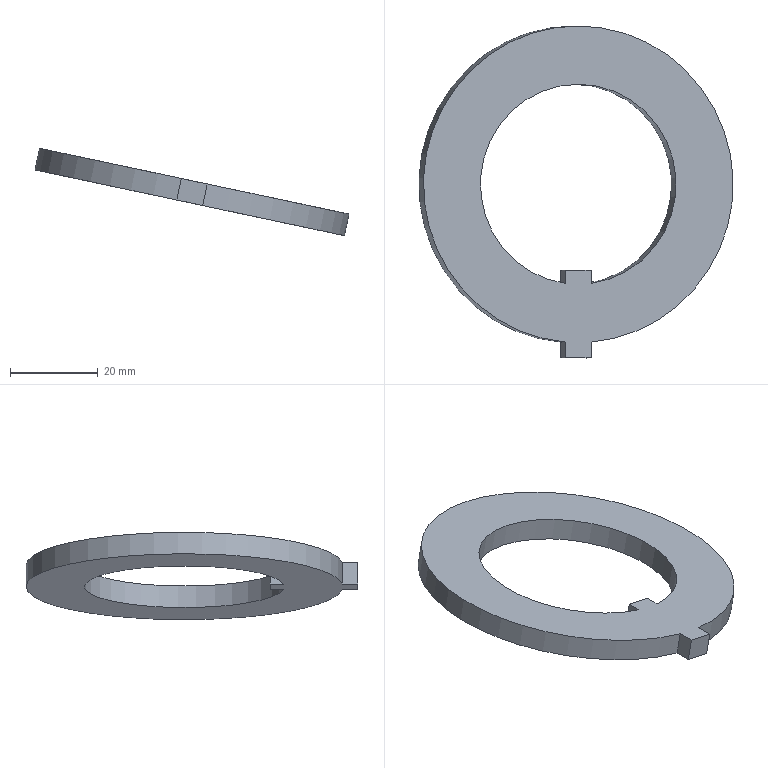Part | STEP file | HL4GZ-1.862.566 (lock washer) | 1 solid | 10 faces | box 71.466 x 75.5 x 19.86 mm | volume 12429 mm3 | plane 8 | cylinder 2 | commonest cylinder face diameters 45.5 x1 72 x1
STEP:
#1=CARTESIAN_POINT('',(0.,0.,0.));
#2=DIRECTION('',(0.,0.,1.));
#3=DIRECTION('',(1.,0.,0.));
#4=AXIS2_PLACEMENT_3D('',#1,#2,#3);
#5=CARTESIAN_POINT('',(1982.907,-35.875,-340.395));
#6=VERTEX_POINT('',#5);
#7=CARTESIAN_POINT('',(1983.947,-35.875,-335.504));
#8=VERTEX_POINT('',#7);
#9=CARTESIAN_POINT('',(1983.947,-35.875,-335.504));
#10=DIRECTION('',(0.2079,0.,0.9781));
#11=VECTOR('',#10,1.);
#12=LINE('',#9,#11);
#13=CARTESIAN_POINT('',(1983.947,-19.5,-335.504));
#14=DIRECTION('',(0.9781,0.,-0.2079));
#15=DIRECTION('',(0.,-1.,0.));
#16=AXIS2_PLACEMENT_3D('',#13,#14,#15);
#17=PLANE('',#16);
#18=CARTESIAN_POINT('',(16.375,0.));
#19=DIRECTION('',(0.,-1.));
#20=VECTOR('',#19,1.);
#21=LINE('',#18,#20);
#22=(GEOMETRIC_REPRESENTATION_CONTEXT(2)PARAMETRIC_REPRESENTATION_CONTEXT()REPRESENTATION_CONTEXT('',''));
#23=DEFINITIONAL_REPRESENTATION('',(#21),#22);
#24=PCURVE('',#17,#23);
#25=CARTESIAN_POINT('',(1981.013,0.00003081,-334.881));
#26=DIRECTION('',(-0.2079,0.,-0.9781));
#27=DIRECTION('',(0.,-1.,0.));
#28=AXIS2_PLACEMENT_3D('',#25,#26,#27);
#29=CYLINDRICAL_SURFACE('',#28,36.);
#30=CARTESIAN_POINT('',(6.2,0.));
#31=DIRECTION('',(0.,-1.));
#32=VECTOR('',#31,1.);
#33=LINE('',#30,#32);
#34=(GEOMETRIC_REPRESENTATION_CONTEXT(2)PARAMETRIC_REPRESENTATION_CONTEXT()REPRESENTATION_CONTEXT('',''));
#35=DEFINITIONAL_REPRESENTATION('',(#33),#34);
#36=PCURVE('',#29,#35);
#37=SURFACE_CURVE('',#12,(#24,#36),.PCURVE_S1.);
#38=EDGE_CURVE('',#6,#8,#37,.T.);
#39=ORIENTED_EDGE('',*,*,#38,.T.);
#40=CARTESIAN_POINT('',(1983.947,-39.5,-335.504));
#41=VERTEX_POINT('',#40);
#42=CARTESIAN_POINT('',(1983.947,-19.5,-335.504));
#43=DIRECTION('',(0.,-1.,0.));
#44=VECTOR('',#43,1.);
#45=LINE('',#42,#44);
#46=CARTESIAN_POINT('',(0.,0.));
#47=DIRECTION('',(1.,0.));
#48=VECTOR('',#47,1.);
#49=LINE('',#46,#48);
#50=(GEOMETRIC_REPRESENTATION_CONTEXT(2)PARAMETRIC_REPRESENTATION_CONTEXT()REPRESENTATION_CONTEXT('',''));
#51=DEFINITIONAL_REPRESENTATION('',(#49),#50);
#52=PCURVE('',#17,#51);
#53=CARTESIAN_POINT('',(1981.013,-29.5,-334.881));
#54=DIRECTION('',(0.2079,0.,0.9781));
#55=DIRECTION('',(-0.9781,0.,0.2079));
#56=AXIS2_PLACEMENT_3D('',#53,#54,#55);
#57=PLANE('',#56);
#58=CARTESIAN_POINT('',(-3.,-10.));
#59=DIRECTION('',(0.,1.));
#60=VECTOR('',#59,1.);
#61=LINE('',#58,#60);
#62=(GEOMETRIC_REPRESENTATION_CONTEXT(2)PARAMETRIC_REPRESENTATION_CONTEXT()REPRESENTATION_CONTEXT('',''));
#63=DEFINITIONAL_REPRESENTATION('',(#61),#62);
#64=PCURVE('',#57,#63);
#65=SURFACE_CURVE('',#45,(#52,#64),.PCURVE_S1.);
#66=EDGE_CURVE('',#8,#41,#65,.T.);
#67=ORIENTED_EDGE('',*,*,#66,.T.);
#68=CARTESIAN_POINT('',(1982.907,-39.5,-340.395));
#69=VERTEX_POINT('',#68);
#70=CARTESIAN_POINT('',(1983.947,-39.5,-335.504));
#71=DIRECTION('',(-0.2079,0.,-0.9781));
#72=VECTOR('',#71,1.);
#73=LINE('',#70,#72);
#74=CARTESIAN_POINT('',(20.,0.));
#75=DIRECTION('',(0.,1.));
#76=VECTOR('',#75,1.);
#77=LINE('',#74,#76);
#78=(GEOMETRIC_REPRESENTATION_CONTEXT(2)PARAMETRIC_REPRESENTATION_CONTEXT()REPRESENTATION_CONTEXT('',''));
#79=DEFINITIONAL_REPRESENTATION('',(#77),#78);
#80=PCURVE('',#17,#79);
#81=CARTESIAN_POINT('',(1983.947,-39.5,-335.504));
#82=DIRECTION('',(0.,-1.,0.));
#83=DIRECTION('',(-0.9781,0.,0.2079));
#84=AXIS2_PLACEMENT_3D('',#81,#82,#83);
#85=PLANE('',#84);
#86=CARTESIAN_POINT('',(0.,0.));
#87=DIRECTION('',(0.,1.));
#88=VECTOR('',#87,1.);
#89=LINE('',#86,#88);
#90=(GEOMETRIC_REPRESENTATION_CONTEXT(2)PARAMETRIC_REPRESENTATION_CONTEXT()REPRESENTATION_CONTEXT('',''));
#91=DEFINITIONAL_REPRESENTATION('',(#89),#90);
#92=PCURVE('',#85,#91);
#93=SURFACE_CURVE('',#73,(#80,#92),.PCURVE_S1.);
#94=EDGE_CURVE('',#41,#69,#93,.T.);
#95=ORIENTED_EDGE('',*,*,#94,.T.);
#96=CARTESIAN_POINT('',(1982.907,-19.5,-340.395));
#97=DIRECTION('',(0.,-1.,0.));
#98=VECTOR('',#97,1.);
#99=LINE('',#96,#98);
#100=CARTESIAN_POINT('',(0.,5.));
#101=DIRECTION('',(1.,0.));
#102=VECTOR('',#101,1.);
#103=LINE('',#100,#102);
#104=(GEOMETRIC_REPRESENTATION_CONTEXT(2)PARAMETRIC_REPRESENTATION_CONTEXT()REPRESENTATION_CONTEXT('',''));
#105=DEFINITIONAL_REPRESENTATION('',(#103),#104);
#106=PCURVE('',#17,#105);
#107=CARTESIAN_POINT('',(1979.973,0.00003081,-339.771));
#108=DIRECTION('',(-0.2079,0.,-0.9781));
#109=DIRECTION('',(0.9781,0.,-0.2079));
#110=AXIS2_PLACEMENT_3D('',#107,#108,#109);
#111=PLANE('',#110);
#112=CARTESIAN_POINT('',(3.,19.5));
#113=DIRECTION('',(0.,1.));
#114=VECTOR('',#113,1.);
#115=LINE('',#112,#114);
#116=(GEOMETRIC_REPRESENTATION_CONTEXT(2)PARAMETRIC_REPRESENTATION_CONTEXT()REPRESENTATION_CONTEXT('',''));
#117=DEFINITIONAL_REPRESENTATION('',(#115),#116);
#118=PCURVE('',#111,#117);
#119=SURFACE_CURVE('',#99,(#106,#118),.PCURVE_S1.);
#120=EDGE_CURVE('',#6,#69,#119,.T.);
#121=ORIENTED_EDGE('',*,*,#120,.F.);
#122=EDGE_LOOP('',(#39,#67,#95,#121));
#123=FACE_BOUND('',#122,.T.);
#124=ADVANCED_FACE('',(#123),#17,.T.);
#125=CARTESIAN_POINT('',(1978.078,-39.5,-334.257));
#126=VERTEX_POINT('',#125);
#127=CARTESIAN_POINT('',(1983.947,-39.5,-335.504));
#128=DIRECTION('',(-0.9781,0.,0.2079));
#129=VECTOR('',#128,1.);
#130=LINE('',#127,#129);
#131=CARTESIAN_POINT('',(0.,0.));
#132=DIRECTION('',(1.,0.));
#133=VECTOR('',#132,1.);
#134=LINE('',#131,#133);
#135=(GEOMETRIC_REPRESENTATION_CONTEXT(2)PARAMETRIC_REPRESENTATION_CONTEXT()REPRESENTATION_CONTEXT('',''));
#136=DEFINITIONAL_REPRESENTATION('',(#134),#135);
#137=PCURVE('',#85,#136);
#138=CARTESIAN_POINT('',(-3.,10.));
#139=DIRECTION('',(1.,0.));
#140=VECTOR('',#139,1.);
#141=LINE('',#138,#140);
#142=(GEOMETRIC_REPRESENTATION_CONTEXT(2)PARAMETRIC_REPRESENTATION_CONTEXT()REPRESENTATION_CONTEXT('',''));
#143=DEFINITIONAL_REPRESENTATION('',(#141),#142);
#144=PCURVE('',#57,#143);
#145=SURFACE_CURVE('',#130,(#137,#144),.PCURVE_S1.);
#146=EDGE_CURVE('',#41,#126,#145,.T.);
#147=ORIENTED_EDGE('',*,*,#146,.T.);
#148=CARTESIAN_POINT('',(1977.039,-39.5,-339.148));
#149=VERTEX_POINT('',#148);
#150=CARTESIAN_POINT('',(1978.078,-39.5,-334.257));
#151=DIRECTION('',(-0.2079,0.,-0.9781));
#152=VECTOR('',#151,1.);
#153=LINE('',#150,#152);
#154=CARTESIAN_POINT('',(6.,0.));
#155=DIRECTION('',(0.,1.));
#156=VECTOR('',#155,1.);
#157=LINE('',#154,#156);
#158=(GEOMETRIC_REPRESENTATION_CONTEXT(2)PARAMETRIC_REPRESENTATION_CONTEXT()REPRESENTATION_CONTEXT('',''));
#159=DEFINITIONAL_REPRESENTATION('',(#157),#158);
#160=PCURVE('',#85,#159);
#161=CARTESIAN_POINT('',(1978.078,-39.5,-334.257));
#162=DIRECTION('',(-0.9781,0.,0.2079));
#163=DIRECTION('',(0.,1.,0.));
#164=AXIS2_PLACEMENT_3D('',#161,#162,#163);
#165=PLANE('',#164);
#166=CARTESIAN_POINT('',(0.,0.));
#167=DIRECTION('',(0.,1.));
#168=VECTOR('',#167,1.);
#169=LINE('',#166,#168);
#170=(GEOMETRIC_REPRESENTATION_CONTEXT(2)PARAMETRIC_REPRESENTATION_CONTEXT()REPRESENTATION_CONTEXT('',''));
#171=DEFINITIONAL_REPRESENTATION('',(#169),#170);
#172=PCURVE('',#165,#171);
#173=SURFACE_CURVE('',#153,(#160,#172),.PCURVE_S1.);
#174=EDGE_CURVE('',#126,#149,#173,.T.);
#175=ORIENTED_EDGE('',*,*,#174,.T.);
#176=CARTESIAN_POINT('',(1982.907,-39.5,-340.395));
#177=DIRECTION('',(-0.9781,0.,0.2079));
#178=VECTOR('',#177,1.);
#179=LINE('',#176,#178);
#180=CARTESIAN_POINT('',(0.,5.));
#181=DIRECTION('',(1.,0.));
#182=VECTOR('',#181,1.);
#183=LINE('',#180,#182);
#184=(GEOMETRIC_REPRESENTATION_CONTEXT(2)PARAMETRIC_REPRESENTATION_CONTEXT()REPRESENTATION_CONTEXT('',''));
#185=DEFINITIONAL_REPRESENTATION('',(#183),#184);
#186=PCURVE('',#85,#185);
#187=CARTESIAN_POINT('',(3.,39.5));
#188=DIRECTION('',(-1.,0.));
#189=VECTOR('',#188,1.);
#190=LINE('',#187,#189);
#191=(GEOMETRIC_REPRESENTATION_CONTEXT(2)PARAMETRIC_REPRESENTATION_CONTEXT()REPRESENTATION_CONTEXT('',''));
#192=DEFINITIONAL_REPRESENTATION('',(#190),#191);
#193=PCURVE('',#111,#192);
#194=SURFACE_CURVE('',#179,(#186,#193),.PCURVE_S1.);
#195=EDGE_CURVE('',#69,#149,#194,.T.);
#196=ORIENTED_EDGE('',*,*,#195,.F.);
#197=ORIENTED_EDGE('',*,*,#94,.F.);
#198=EDGE_LOOP('',(#147,#175,#196,#197));
#199=FACE_BOUND('',#198,.T.);
#200=ADVANCED_FACE('',(#199),#85,.T.);
#201=CARTESIAN_POINT('',(1978.078,-22.551,-334.257));
#202=VERTEX_POINT('',#201);
#203=CARTESIAN_POINT('',(1977.039,-22.551,-339.148));
#204=VERTEX_POINT('',#203);
#205=CARTESIAN_POINT('',(1978.078,-22.551,-334.257));
#206=DIRECTION('',(-0.2079,0.,-0.9781));
#207=VECTOR('',#206,1.);
#208=LINE('',#205,#207);
#209=CARTESIAN_POINT('',(1978.078,-39.5,-334.257));
#210=DIRECTION('',(-0.9781,0.,0.2079));
#211=DIRECTION('',(0.,1.,0.));
#212=AXIS2_PLACEMENT_3D('',#209,#210,#211);
#213=PLANE('',#212);
#214=CARTESIAN_POINT('',(16.949,0.));
#215=DIRECTION('',(0.,1.));
#216=VECTOR('',#215,1.);
#217=LINE('',#214,#216);
#218=(GEOMETRIC_REPRESENTATION_CONTEXT(2)PARAMETRIC_REPRESENTATION_CONTEXT()REPRESENTATION_CONTEXT('',''));
#219=DEFINITIONAL_REPRESENTATION('',(#217),#218);
#220=PCURVE('',#213,#219);
#221=CARTESIAN_POINT('',(1981.013,0.00003081,-334.881));
#222=DIRECTION('',(-0.2079,0.,-0.9781));
#223=DIRECTION('',(0.,-1.,0.));
#224=AXIS2_PLACEMENT_3D('',#221,#222,#223);
#225=CYLINDRICAL_SURFACE('',#224,22.75);
#226=CARTESIAN_POINT('',(0.1323,0.));
#227=DIRECTION('',(0.,1.));
#228=VECTOR('',#227,1.);
#229=LINE('',#226,#228);
#230=(GEOMETRIC_REPRESENTATION_CONTEXT(2)PARAMETRIC_REPRESENTATION_CONTEXT()REPRESENTATION_CONTEXT('',''));
#231=DEFINITIONAL_REPRESENTATION('',(#229),#230);
#232=PCURVE('',#225,#231);
#233=SURFACE_CURVE('',#208,(#220,#232),.PCURVE_S1.);
#234=EDGE_CURVE('',#202,#204,#233,.T.);
#235=ORIENTED_EDGE('',*,*,#234,.F.);
#236=CARTESIAN_POINT('',(1978.078,-19.5,-334.257));
#237=VERTEX_POINT('',#236);
#238=CARTESIAN_POINT('',(1978.078,-39.5,-334.257));
#239=DIRECTION('',(0.,1.,0.));
#240=VECTOR('',#239,1.);
#241=LINE('',#238,#240);
#242=CARTESIAN_POINT('',(0.,0.));
#243=DIRECTION('',(1.,0.));
#244=VECTOR('',#243,1.);
#245=LINE('',#242,#244);
#246=(GEOMETRIC_REPRESENTATION_CONTEXT(2)PARAMETRIC_REPRESENTATION_CONTEXT()REPRESENTATION_CONTEXT('',''));
#247=DEFINITIONAL_REPRESENTATION('',(#245),#246);
#248=PCURVE('',#213,#247);
#249=CARTESIAN_POINT('',(3.,10.));
#250=DIRECTION('',(0.,-1.));
#251=VECTOR('',#250,1.);
#252=LINE('',#249,#251);
#253=(GEOMETRIC_REPRESENTATION_CONTEXT(2)PARAMETRIC_REPRESENTATION_CONTEXT()REPRESENTATION_CONTEXT('',''));
#254=DEFINITIONAL_REPRESENTATION('',(#252),#253);
#255=PCURVE('',#57,#254);
#256=SURFACE_CURVE('',#241,(#248,#255),.PCURVE_S1.);
#257=EDGE_CURVE('',#202,#237,#256,.T.);
#258=ORIENTED_EDGE('',*,*,#257,.T.);
#259=CARTESIAN_POINT('',(1977.039,-19.5,-339.148));
#260=VERTEX_POINT('',#259);
#261=CARTESIAN_POINT('',(1978.078,-19.5,-334.257));
#262=DIRECTION('',(-0.2079,0.,-0.9781));
#263=VECTOR('',#262,1.);
#264=LINE('',#261,#263);
#265=CARTESIAN_POINT('',(20.,0.));
#266=DIRECTION('',(0.,1.));
#267=VECTOR('',#266,1.);
#268=LINE('',#265,#267);
#269=(GEOMETRIC_REPRESENTATION_CONTEXT(2)PARAMETRIC_REPRESENTATION_CONTEXT()REPRESENTATION_CONTEXT('',''));
#270=DEFINITIONAL_REPRESENTATION('',(#268),#269);
#271=PCURVE('',#213,#270);
#272=CARTESIAN_POINT('',(1978.078,-19.5,-334.257));
#273=DIRECTION('',(0.,1.,0.));
#274=DIRECTION('',(0.9781,0.,-0.2079));
#275=AXIS2_PLACEMENT_3D('',#272,#273,#274);
#276=PLANE('',#275);
#277=CARTESIAN_POINT('',(0.,0.));
#278=DIRECTION('',(0.,1.));
#279=VECTOR('',#278,1.);
#280=LINE('',#277,#279);
#281=(GEOMETRIC_REPRESENTATION_CONTEXT(2)PARAMETRIC_REPRESENTATION_CONTEXT()REPRESENTATION_CONTEXT('',''));
#282=DEFINITIONAL_REPRESENTATION('',(#280),#281);
#283=PCURVE('',#276,#282);
#284=SURFACE_CURVE('',#264,(#271,#283),.PCURVE_S1.);
#285=EDGE_CURVE('',#237,#260,#284,.T.);
#286=ORIENTED_EDGE('',*,*,#285,.T.);
#287=CARTESIAN_POINT('',(1977.039,-39.5,-339.148));
#288=DIRECTION('',(0.,1.,0.));
#289=VECTOR('',#288,1.);
#290=LINE('',#287,#289);
#291=CARTESIAN_POINT('',(0.,5.));
#292=DIRECTION('',(1.,0.));
#293=VECTOR('',#292,1.);
#294=LINE('',#291,#293);
#295=(GEOMETRIC_REPRESENTATION_CONTEXT(2)PARAMETRIC_REPRESENTATION_CONTEXT()REPRESENTATION_CONTEXT('',''));
#296=DEFINITIONAL_REPRESENTATION('',(#294),#295);
#297=PCURVE('',#213,#296);
#298=CARTESIAN_POINT('',(-3.,39.5));
#299=DIRECTION('',(0.,-1.));
#300=VECTOR('',#299,1.);
#301=LINE('',#298,#300);
#302=(GEOMETRIC_REPRESENTATION_CONTEXT(2)PARAMETRIC_REPRESENTATION_CONTEXT()REPRESENTATION_CONTEXT('',''));
#303=DEFINITIONAL_REPRESENTATION('',(#301),#302);
#304=PCURVE('',#111,#303);
#305=SURFACE_CURVE('',#290,(#297,#304),.PCURVE_S1.);
#306=EDGE_CURVE('',#204,#260,#305,.T.);
#307=ORIENTED_EDGE('',*,*,#306,.F.);
#308=EDGE_LOOP('',(#235,#258,#286,#307));
#309=FACE_BOUND('',#308,.T.);
#310=ADVANCED_FACE('',(#309),#213,.T.);
#311=CARTESIAN_POINT('',(1983.947,-19.5,-335.504));
#312=VERTEX_POINT('',#311);
#313=CARTESIAN_POINT('',(1978.078,-19.5,-334.257));
#314=DIRECTION('',(0.9781,0.,-0.2079));
#315=VECTOR('',#314,1.);
#316=LINE('',#313,#315);
#317=CARTESIAN_POINT('',(0.,0.));
#318=DIRECTION('',(1.,0.));
#319=VECTOR('',#318,1.);
#320=LINE('',#317,#319);
#321=(GEOMETRIC_REPRESENTATION_CONTEXT(2)PARAMETRIC_REPRESENTATION_CONTEXT()REPRESENTATION_CONTEXT('',''));
#322=DEFINITIONAL_REPRESENTATION('',(#320),#321);
#323=PCURVE('',#276,#322);
#324=CARTESIAN_POINT('',(3.,-10.));
#325=DIRECTION('',(-1.,0.));
#326=VECTOR('',#325,1.);
#327=LINE('',#324,#326);
#328=(GEOMETRIC_REPRESENTATION_CONTEXT(2)PARAMETRIC_REPRESENTATION_CONTEXT()REPRESENTATION_CONTEXT('',''));
#329=DEFINITIONAL_REPRESENTATION('',(#327),#328);
#330=PCURVE('',#57,#329);
#331=SURFACE_CURVE('',#316,(#323,#330),.PCURVE_S1.);
#332=EDGE_CURVE('',#237,#312,#331,.T.);
#333=ORIENTED_EDGE('',*,*,#332,.T.);
#334=CARTESIAN_POINT('',(1982.907,-19.5,-340.395));
#335=VERTEX_POINT('',#334);
#336=CARTESIAN_POINT('',(1983.947,-19.5,-335.504));
#337=DIRECTION('',(-0.2079,0.,-0.9781));
#338=VECTOR('',#337,1.);
#339=LINE('',#336,#338);
#340=CARTESIAN_POINT('',(6.,0.));
#341=DIRECTION('',(0.,1.));
#342=VECTOR('',#341,1.);
#343=LINE('',#340,#342);
#344=(GEOMETRIC_REPRESENTATION_CONTEXT(2)PARAMETRIC_REPRESENTATION_CONTEXT()REPRESENTATION_CONTEXT('',''));
#345=DEFINITIONAL_REPRESENTATION('',(#343),#344);
#346=PCURVE('',#276,#345);
#347=CARTESIAN_POINT('',(1983.947,-19.5,-335.504));
#348=DIRECTION('',(0.9781,0.,-0.2079));
#349=DIRECTION('',(0.,-1.,0.));
#350=AXIS2_PLACEMENT_3D('',#347,#348,#349);
#351=PLANE('',#350);
#352=CARTESIAN_POINT('',(0.,0.));
#353=DIRECTION('',(0.,1.));
#354=VECTOR('',#353,1.);
#355=LINE('',#352,#354);
#356=(GEOMETRIC_REPRESENTATION_CONTEXT(2)PARAMETRIC_REPRESENTATION_CONTEXT()REPRESENTATION_CONTEXT('',''));
#357=DEFINITIONAL_REPRESENTATION('',(#355),#356);
#358=PCURVE('',#351,#357);
#359=SURFACE_CURVE('',#339,(#346,#358),.PCURVE_S1.);
#360=EDGE_CURVE('',#312,#335,#359,.T.);
#361=ORIENTED_EDGE('',*,*,#360,.T.);
#362=CARTESIAN_POINT('',(1977.039,-19.5,-339.148));
#363=DIRECTION('',(0.9781,0.,-0.2079));
#364=VECTOR('',#363,1.);
#365=LINE('',#362,#364);
#366=CARTESIAN_POINT('',(0.,5.));
#367=DIRECTION('',(1.,0.));
#368=VECTOR('',#367,1.);
#369=LINE('',#366,#368);
#370=(GEOMETRIC_REPRESENTATION_CONTEXT(2)PARAMETRIC_REPRESENTATION_CONTEXT()REPRESENTATION_CONTEXT('',''));
#371=DEFINITIONAL_REPRESENTATION('',(#369),#370);
#372=PCURVE('',#276,#371);
#373=CARTESIAN_POINT('',(-3.,19.5));
#374=DIRECTION('',(1.,0.));
#375=VECTOR('',#374,1.);
#376=LINE('',#373,#375);
#377=(GEOMETRIC_REPRESENTATION_CONTEXT(2)PARAMETRIC_REPRESENTATION_CONTEXT()REPRESENTATION_CONTEXT('',''));
#378=DEFINITIONAL_REPRESENTATION('',(#376),#377);
#379=PCURVE('',#111,#378);
#380=SURFACE_CURVE('',#365,(#372,#379),.PCURVE_S1.);
#381=EDGE_CURVE('',#260,#335,#380,.T.);
#382=ORIENTED_EDGE('',*,*,#381,.F.);
#383=ORIENTED_EDGE('',*,*,#285,.F.);
#384=EDGE_LOOP('',(#333,#361,#382,#383));
#385=FACE_BOUND('',#384,.T.);
#386=ADVANCED_FACE('',(#385),#276,.T.);
#387=CARTESIAN_POINT('',(1978.078,-35.875,-334.257));
#388=VERTEX_POINT('',#387);
#389=CARTESIAN_POINT('',(1977.039,-35.875,-339.148));
#390=VERTEX_POINT('',#389);
#391=CARTESIAN_POINT('',(1978.078,-35.875,-334.257));
#392=DIRECTION('',(-0.2079,0.,-0.9781));
#393=VECTOR('',#392,1.);
#394=LINE('',#391,#393);
#395=CARTESIAN_POINT('',(3.625,0.));
#396=DIRECTION('',(0.,1.));
#397=VECTOR('',#396,1.);
#398=LINE('',#395,#397);
#399=(GEOMETRIC_REPRESENTATION_CONTEXT(2)PARAMETRIC_REPRESENTATION_CONTEXT()REPRESENTATION_CONTEXT('',''));
#400=DEFINITIONAL_REPRESENTATION('',(#398),#399);
#401=PCURVE('',#165,#400);
#402=CARTESIAN_POINT('',(0.08343,0.));
#403=DIRECTION('',(0.,1.));
#404=VECTOR('',#403,1.);
#405=LINE('',#402,#404);
#406=(GEOMETRIC_REPRESENTATION_CONTEXT(2)PARAMETRIC_REPRESENTATION_CONTEXT()REPRESENTATION_CONTEXT('',''));
#407=DEFINITIONAL_REPRESENTATION('',(#405),#406);
#408=PCURVE('',#29,#407);
#409=SURFACE_CURVE('',#394,(#401,#408),.PCURVE_S1.);
#410=EDGE_CURVE('',#388,#390,#409,.T.);
#411=ORIENTED_EDGE('',*,*,#410,.T.);
#412=CARTESIAN_POINT('',(1977.039,-39.5,-339.148));
#413=DIRECTION('',(0.,1.,0.));
#414=VECTOR('',#413,1.);
#415=LINE('',#412,#414);
#416=CARTESIAN_POINT('',(0.,5.));
#417=DIRECTION('',(1.,0.));
#418=VECTOR('',#417,1.);
#419=LINE('',#416,#418);
#420=(GEOMETRIC_REPRESENTATION_CONTEXT(2)PARAMETRIC_REPRESENTATION_CONTEXT()REPRESENTATION_CONTEXT('',''));
#421=DEFINITIONAL_REPRESENTATION('',(#419),#420);
#422=PCURVE('',#165,#421);
#423=CARTESIAN_POINT('',(-3.,39.5));
#424=DIRECTION('',(0.,-1.));
#425=VECTOR('',#424,1.);
#426=LINE('',#423,#425);
#427=(GEOMETRIC_REPRESENTATION_CONTEXT(2)PARAMETRIC_REPRESENTATION_CONTEXT()REPRESENTATION_CONTEXT('',''));
#428=DEFINITIONAL_REPRESENTATION('',(#426),#427);
#429=PCURVE('',#111,#428);
#430=SURFACE_CURVE('',#415,(#422,#429),.PCURVE_S1.);
#431=EDGE_CURVE('',#149,#390,#430,.T.);
#432=ORIENTED_EDGE('',*,*,#431,.F.);
#433=ORIENTED_EDGE('',*,*,#174,.F.);
#434=CARTESIAN_POINT('',(1978.078,-39.5,-334.257));
#435=DIRECTION('',(0.,1.,0.));
#436=VECTOR('',#435,1.);
#437=LINE('',#434,#436);
#438=CARTESIAN_POINT('',(0.,0.));
#439=DIRECTION('',(1.,0.));
#440=VECTOR('',#439,1.);
#441=LINE('',#438,#440);
#442=(GEOMETRIC_REPRESENTATION_CONTEXT(2)PARAMETRIC_REPRESENTATION_CONTEXT()REPRESENTATION_CONTEXT('',''));
#443=DEFINITIONAL_REPRESENTATION('',(#441),#442);
#444=PCURVE('',#165,#443);
#445=CARTESIAN_POINT('',(3.,10.));
#446=DIRECTION('',(0.,-1.));
#447=VECTOR('',#446,1.);
#448=LINE('',#445,#447);
#449=(GEOMETRIC_REPRESENTATION_CONTEXT(2)PARAMETRIC_REPRESENTATION_CONTEXT()REPRESENTATION_CONTEXT('',''));
#450=DEFINITIONAL_REPRESENTATION('',(#448),#449);
#451=PCURVE('',#57,#450);
#452=SURFACE_CURVE('',#437,(#444,#451),.PCURVE_S1.);
#453=EDGE_CURVE('',#126,#388,#452,.T.);
#454=ORIENTED_EDGE('',*,*,#453,.T.);
#455=EDGE_LOOP('',(#411,#432,#433,#454));
#456=FACE_BOUND('',#455,.T.);
#457=ADVANCED_FACE('',(#456),#165,.T.);
#458=CARTESIAN_POINT('',(1983.947,-22.551,-335.504));
#459=VERTEX_POINT('',#458);
#460=CARTESIAN_POINT('',(1983.947,-19.5,-335.504));
#461=DIRECTION('',(0.,-1.,0.));
#462=VECTOR('',#461,1.);
#463=LINE('',#460,#462);
#464=CARTESIAN_POINT('',(-3.,-10.));
#465=DIRECTION('',(0.,1.));
#466=VECTOR('',#465,1.);
#467=LINE('',#464,#466);
#468=(GEOMETRIC_REPRESENTATION_CONTEXT(2)PARAMETRIC_REPRESENTATION_CONTEXT()REPRESENTATION_CONTEXT('',''));
#469=DEFINITIONAL_REPRESENTATION('',(#467),#468);
#470=PCURVE('',#57,#469);
#471=CARTESIAN_POINT('',(0.,0.));
#472=DIRECTION('',(1.,0.));
#473=VECTOR('',#472,1.);
#474=LINE('',#471,#473);
#475=(GEOMETRIC_REPRESENTATION_CONTEXT(2)PARAMETRIC_REPRESENTATION_CONTEXT()REPRESENTATION_CONTEXT('',''));
#476=DEFINITIONAL_REPRESENTATION('',(#474),#475);
#477=PCURVE('',#351,#476);
#478=SURFACE_CURVE('',#463,(#470,#477),.PCURVE_S1.);
#479=EDGE_CURVE('',#312,#459,#478,.T.);
#480=ORIENTED_EDGE('',*,*,#479,.F.);
#481=ORIENTED_EDGE('',*,*,#332,.F.);
#482=ORIENTED_EDGE('',*,*,#257,.F.);
#483=CARTESIAN_POINT('',(1981.013,0.00003081,-334.881));
#484=DIRECTION('',(-0.2079,0.,-0.9781));
#485=DIRECTION('',(0.,-1.,0.));
#486=AXIS2_PLACEMENT_3D('',#483,#484,#485);
#487=CIRCLE('',#486,22.75);
#488=CARTESIAN_POINT('',(0.,-6.75));
#489=CARTESIAN_POINT('',(39.404,-6.75));
#490=CARTESIAN_POINT('',(19.702,-40.875));
#491=CARTESIAN_POINT('',(0.,-75.));
#492=CARTESIAN_POINT('',(-19.702,-40.875));
#493=CARTESIAN_POINT('',(-39.404,-6.75));
#494=CARTESIAN_POINT('',(0.,-6.75));
#495=(BOUNDED_CURVE()B_SPLINE_CURVE(2,(#488,#489,#490,#491,#492,#493,#494),.UNSPECIFIED.,.T.,.F.)B_SPLINE_CURVE_WITH_KNOTS((1,2,2,2,2,1),(-2.094,0.,2.094,4.189,6.283,8.378),.UNSPECIFIED.)CURVE()GEOMETRIC_REPRESENTATION_ITEM()RATIONAL_B_SPLINE_CURVE((1.,0.5,1.,0.5,1.,0.5,1.))REPRESENTATION_ITEM(''));
#496=(GEOMETRIC_REPRESENTATION_CONTEXT(2)PARAMETRIC_REPRESENTATION_CONTEXT()REPRESENTATION_CONTEXT('',''));
#497=DEFINITIONAL_REPRESENTATION('',(#495),#496);
#498=PCURVE('',#57,#497);
#499=CARTESIAN_POINT('',(0.,0.));
#500=DIRECTION('',(1.,0.));
#501=VECTOR('',#500,1.);
#502=LINE('',#499,#501);
#503=(GEOMETRIC_REPRESENTATION_CONTEXT(2)PARAMETRIC_REPRESENTATION_CONTEXT()REPRESENTATION_CONTEXT('',''));
#504=DEFINITIONAL_REPRESENTATION('',(#502),#503);
#505=PCURVE('',#225,#504);
#506=SURFACE_CURVE('',#487,(#498,#505),.PCURVE_S1.);
#507=EDGE_CURVE('',#202,#459,#506,.T.);
#508=ORIENTED_EDGE('',*,*,#507,.T.);
#509=EDGE_LOOP('',(#480,#481,#482,#508));
#510=FACE_BOUND('',#509,.T.);
#511=CARTESIAN_POINT('',(1981.013,0.00003081,-334.881));
#512=DIRECTION('',(0.2079,0.,0.9781));
#513=DIRECTION('',(0.,-1.,0.));
#514=AXIS2_PLACEMENT_3D('',#511,#512,#513);
#515=CIRCLE('',#514,36.);
#516=CARTESIAN_POINT('',(0.,-29.5));
#517=DIRECTION('',(0.,1.));
#518=AXIS2_PLACEMENT_2D('',#516,#517);
#519=CIRCLE('',#518,36.);
#520=(GEOMETRIC_REPRESENTATION_CONTEXT(2)PARAMETRIC_REPRESENTATION_CONTEXT()REPRESENTATION_CONTEXT('',''));
#521=DEFINITIONAL_REPRESENTATION('',(#519),#520);
#522=PCURVE('',#57,#521);
#523=CARTESIAN_POINT('',(6.283,0.));
#524=DIRECTION('',(-1.,0.));
#525=VECTOR('',#524,1.);
#526=LINE('',#523,#525);
#527=(GEOMETRIC_REPRESENTATION_CONTEXT(2)PARAMETRIC_REPRESENTATION_CONTEXT()REPRESENTATION_CONTEXT('',''));
#528=DEFINITIONAL_REPRESENTATION('',(#526),#527);
#529=PCURVE('',#29,#528);
#530=SURFACE_CURVE('',#515,(#522,#529),.PCURVE_S1.);
#531=EDGE_CURVE('',#8,#388,#530,.T.);
#532=ORIENTED_EDGE('',*,*,#531,.T.);
#533=ORIENTED_EDGE('',*,*,#453,.F.);
#534=ORIENTED_EDGE('',*,*,#146,.F.);
#535=ORIENTED_EDGE('',*,*,#66,.F.);
#536=EDGE_LOOP('',(#532,#533,#534,#535));
#537=FACE_BOUND('',#536,.T.);
#538=ADVANCED_FACE('',(#510,#537),#57,.T.);
#539=ORIENTED_EDGE('',*,*,#410,.F.);
#540=ORIENTED_EDGE('',*,*,#531,.F.);
#541=ORIENTED_EDGE('',*,*,#38,.F.);
#542=CARTESIAN_POINT('',(1979.973,0.00003081,-339.771));
#543=DIRECTION('',(-0.2079,0.,-0.9781));
#544=DIRECTION('',(0.,-1.,0.));
#545=AXIS2_PLACEMENT_3D('',#542,#543,#544);
#546=CIRCLE('',#545,36.);
#547=CARTESIAN_POINT('',(0.,5.));
#548=DIRECTION('',(1.,0.));
#549=VECTOR('',#548,1.);
#550=LINE('',#547,#549);
#551=(GEOMETRIC_REPRESENTATION_CONTEXT(2)PARAMETRIC_REPRESENTATION_CONTEXT()REPRESENTATION_CONTEXT('',''));
#552=DEFINITIONAL_REPRESENTATION('',(#550),#551);
#553=PCURVE('',#29,#552);
#554=CARTESIAN_POINT('',(0.,0.));
#555=DIRECTION('',(0.,1.));
#556=AXIS2_PLACEMENT_2D('',#554,#555);
#557=CIRCLE('',#556,36.);
#558=(GEOMETRIC_REPRESENTATION_CONTEXT(2)PARAMETRIC_REPRESENTATION_CONTEXT()REPRESENTATION_CONTEXT('',''));
#559=DEFINITIONAL_REPRESENTATION('',(#557),#558);
#560=PCURVE('',#111,#559);
#561=SURFACE_CURVE('',#546,(#553,#560),.PCURVE_S1.);
#562=EDGE_CURVE('',#390,#6,#561,.T.);
#563=ORIENTED_EDGE('',*,*,#562,.F.);
#564=EDGE_LOOP('',(#539,#540,#541,#563));
#565=FACE_BOUND('',#564,.T.);
#566=ADVANCED_FACE('',(#565),#29,.T.);
#567=CARTESIAN_POINT('',(1982.907,-22.551,-340.395));
#568=VERTEX_POINT('',#567);
#569=CARTESIAN_POINT('',(1979.973,0.00003081,-339.771));
#570=DIRECTION('',(0.2079,0.,0.9781));
#571=DIRECTION('',(0.,-1.,0.));
#572=AXIS2_PLACEMENT_3D('',#569,#570,#571);
#573=CIRCLE('',#572,22.75);
#574=CARTESIAN_POINT('',(0.,22.75));
#575=CARTESIAN_POINT('',(39.404,22.75));
#576=CARTESIAN_POINT('',(19.702,-11.375));
#577=CARTESIAN_POINT('',(0.,-45.5));
#578=CARTESIAN_POINT('',(-19.702,-11.375));
#579=CARTESIAN_POINT('',(-39.404,22.75));
#580=CARTESIAN_POINT('',(0.,22.75));
#581=(BOUNDED_CURVE()B_SPLINE_CURVE(2,(#574,#575,#576,#577,#578,#579,#580),.UNSPECIFIED.,.T.,.F.)B_SPLINE_CURVE_WITH_KNOTS((1,2,2,2,2,1),(-2.094,0.,2.094,4.189,6.283,8.378),.UNSPECIFIED.)CURVE()GEOMETRIC_REPRESENTATION_ITEM()RATIONAL_B_SPLINE_CURVE((1.,0.5,1.,0.5,1.,0.5,1.))REPRESENTATION_ITEM(''));
#582=(GEOMETRIC_REPRESENTATION_CONTEXT(2)PARAMETRIC_REPRESENTATION_CONTEXT()REPRESENTATION_CONTEXT('',''));
#583=DEFINITIONAL_REPRESENTATION('',(#581),#582);
#584=PCURVE('',#111,#583);
#585=CARTESIAN_POINT('',(6.283,5.));
#586=DIRECTION('',(-1.,0.));
#587=VECTOR('',#586,1.);
#588=LINE('',#585,#587);
#589=(GEOMETRIC_REPRESENTATION_CONTEXT(2)PARAMETRIC_REPRESENTATION_CONTEXT()REPRESENTATION_CONTEXT('',''));
#590=DEFINITIONAL_REPRESENTATION('',(#588),#589);
#591=PCURVE('',#225,#590);
#592=SURFACE_CURVE('',#573,(#584,#591),.PCURVE_S1.);
#593=EDGE_CURVE('',#568,#204,#592,.T.);
#594=ORIENTED_EDGE('',*,*,#593,.T.);
#595=ORIENTED_EDGE('',*,*,#306,.T.);
#596=ORIENTED_EDGE('',*,*,#381,.T.);
#597=CARTESIAN_POINT('',(1982.907,-19.5,-340.395));
#598=DIRECTION('',(0.,-1.,0.));
#599=VECTOR('',#598,1.);
#600=LINE('',#597,#599);
#601=CARTESIAN_POINT('',(3.,19.5));
#602=DIRECTION('',(0.,1.));
#603=VECTOR('',#602,1.);
#604=LINE('',#601,#603);
#605=(GEOMETRIC_REPRESENTATION_CONTEXT(2)PARAMETRIC_REPRESENTATION_CONTEXT()REPRESENTATION_CONTEXT('',''));
#606=DEFINITIONAL_REPRESENTATION('',(#604),#605);
#607=PCURVE('',#111,#606);
#608=CARTESIAN_POINT('',(0.,5.));
#609=DIRECTION('',(1.,0.));
#610=VECTOR('',#609,1.);
#611=LINE('',#608,#610);
#612=(GEOMETRIC_REPRESENTATION_CONTEXT(2)PARAMETRIC_REPRESENTATION_CONTEXT()REPRESENTATION_CONTEXT('',''));
#613=DEFINITIONAL_REPRESENTATION('',(#611),#612);
#614=PCURVE('',#351,#613);
#615=SURFACE_CURVE('',#600,(#607,#614),.PCURVE_S1.);
#616=EDGE_CURVE('',#335,#568,#615,.T.);
#617=ORIENTED_EDGE('',*,*,#616,.T.);
#618=EDGE_LOOP('',(#594,#595,#596,#617));
#619=FACE_BOUND('',#618,.T.);
#620=ORIENTED_EDGE('',*,*,#562,.T.);
#621=ORIENTED_EDGE('',*,*,#120,.T.);
#622=ORIENTED_EDGE('',*,*,#195,.T.);
#623=ORIENTED_EDGE('',*,*,#431,.T.);
#624=EDGE_LOOP('',(#620,#621,#622,#623));
#625=FACE_BOUND('',#624,.T.);
#626=ADVANCED_FACE('',(#619,#625),#111,.T.);
#627=CARTESIAN_POINT('',(1983.947,-22.551,-335.504));
#628=DIRECTION('',(0.2079,0.,0.9781));
#629=VECTOR('',#628,1.);
#630=LINE('',#627,#629);
#631=CARTESIAN_POINT('',(3.051,0.));
#632=DIRECTION('',(0.,-1.));
#633=VECTOR('',#632,1.);
#634=LINE('',#631,#633);
#635=(GEOMETRIC_REPRESENTATION_CONTEXT(2)PARAMETRIC_REPRESENTATION_CONTEXT()REPRESENTATION_CONTEXT('',''));
#636=DEFINITIONAL_REPRESENTATION('',(#634),#635);
#637=PCURVE('',#351,#636);
#638=CARTESIAN_POINT('',(6.151,0.));
#639=DIRECTION('',(0.,-1.));
#640=VECTOR('',#639,1.);
#641=LINE('',#638,#640);
#642=(GEOMETRIC_REPRESENTATION_CONTEXT(2)PARAMETRIC_REPRESENTATION_CONTEXT()REPRESENTATION_CONTEXT('',''));
#643=DEFINITIONAL_REPRESENTATION('',(#641),#642);
#644=PCURVE('',#225,#643);
#645=SURFACE_CURVE('',#630,(#637,#644),.PCURVE_S1.);
#646=EDGE_CURVE('',#568,#459,#645,.T.);
#647=ORIENTED_EDGE('',*,*,#646,.F.);
#648=ORIENTED_EDGE('',*,*,#616,.F.);
#649=ORIENTED_EDGE('',*,*,#360,.F.);
#650=ORIENTED_EDGE('',*,*,#479,.T.);
#651=EDGE_LOOP('',(#647,#648,#649,#650));
#652=FACE_BOUND('',#651,.T.);
#653=ADVANCED_FACE('',(#652),#351,.T.);
#654=ORIENTED_EDGE('',*,*,#593,.T.);
#655=ORIENTED_EDGE('',*,*,#234,.F.);
#656=ORIENTED_EDGE('',*,*,#507,.T.);
#657=ORIENTED_EDGE('',*,*,#646,.F.);
#658=EDGE_LOOP('',(#654,#655,#656,#657));
#659=FACE_BOUND('',#658,.F.);
#660=ADVANCED_FACE('',(#659),#225,.F.);
#661=CLOSED_SHELL('',(#124,#200,#310,#386,#457,#538,#566,#626,#653,#660));
#662=MANIFOLD_SOLID_BREP('',#661);
#663=(LENGTH_UNIT()NAMED_UNIT(*)SI_UNIT(.MILLI.,.METRE.));
#664=UNCERTAINTY_MEASURE_WITH_UNIT(LENGTH_MEASURE(0.0000001),#663,'','');
#665=(NAMED_UNIT(*)PLANE_ANGLE_UNIT()SI_UNIT($,.RADIAN.));
#666=(NAMED_UNIT(*)SI_UNIT($,.STERADIAN.)SOLID_ANGLE_UNIT());
#667=(GEOMETRIC_REPRESENTATION_CONTEXT(3)GLOBAL_UNCERTAINTY_ASSIGNED_CONTEXT((#664))GLOBAL_UNIT_ASSIGNED_CONTEXT((#663,#665,#666))REPRESENTATION_CONTEXT('',''));
#668=ADVANCED_BREP_SHAPE_REPRESENTATION('',(#4,#662),#667);